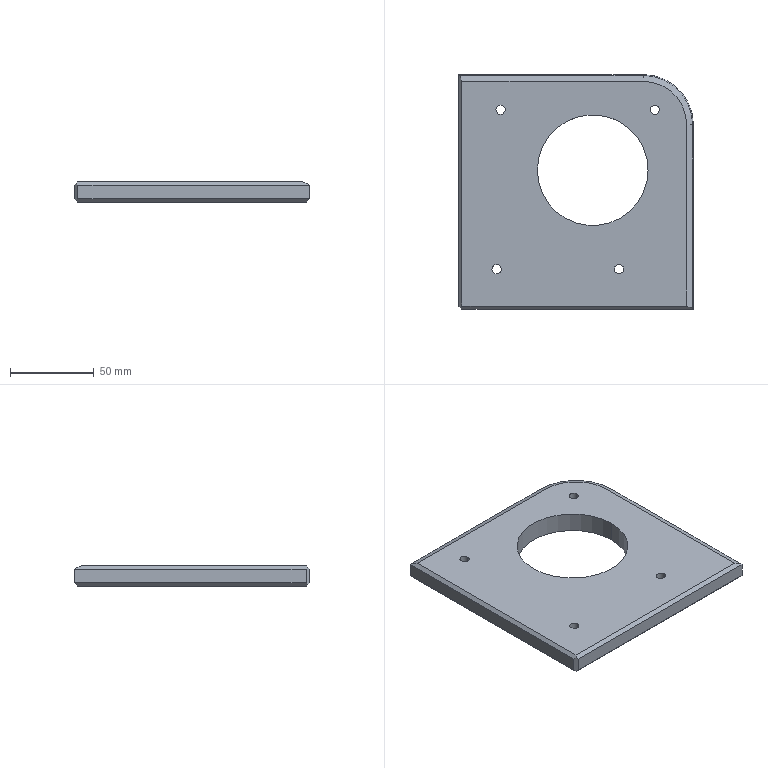Part | Creo | 1 solid | 43 faces | box 140 x 140 x 12 mm | volume 187002 mm3 | plane 21 | cylinder 19 | cone 3 | commonest cylinder face diameters 5.5 x8 9.5 x8 66 x2 60 x1
STEP:
#1=CARTESIAN_POINT('',(-313.,-373.005,1.));
#2=VERTEX_POINT('',#1);
#3=CARTESIAN_POINT('',(-313.,-239.005,1.));
#4=VERTEX_POINT('',#3);
#5=CARTESIAN_POINT('',(-313.,-373.005,1.));
#6=DIRECTION('',(0.,1.,0.));
#7=VECTOR('',#6,134.);
#8=LINE('',#5,#7);
#9=EDGE_CURVE('',#2,#4,#8,.T.);
#10=ORIENTED_EDGE('',*,*,#9,.T.);
#11=CARTESIAN_POINT('',(-205.,-239.005,1.));
#12=VERTEX_POINT('',#11);
#13=CARTESIAN_POINT('',(-313.,-239.005,1.));
#14=DIRECTION('',(1.,0.,0.));
#15=VECTOR('',#14,108.);
#16=LINE('',#13,#15);
#17=EDGE_CURVE('',#4,#12,#16,.T.);
#18=ORIENTED_EDGE('',*,*,#17,.T.);
#19=CARTESIAN_POINT('',(-179.,-265.005,1.));
#20=VERTEX_POINT('',#19);
#21=CARTESIAN_POINT('',(-205.,-265.005,1.));
#22=DIRECTION('',(0.,0.,1.));
#23=DIRECTION('',(1.,0.,0.));
#24=AXIS2_PLACEMENT_3D('',#21,#22,#23);
#25=CIRCLE('',#24,26.);
#26=EDGE_CURVE('',#20,#12,#25,.T.);
#27=ORIENTED_EDGE('',*,*,#26,.F.);
#28=CARTESIAN_POINT('',(-179.,-373.005,1.));
#29=VERTEX_POINT('',#28);
#30=CARTESIAN_POINT('',(-179.,-265.005,1.));
#31=DIRECTION('',(0.,-1.,0.));
#32=VECTOR('',#31,108.);
#33=LINE('',#30,#32);
#34=EDGE_CURVE('',#20,#29,#33,.T.);
#35=ORIENTED_EDGE('',*,*,#34,.T.);
#36=CARTESIAN_POINT('',(-179.,-373.005,1.));
#37=DIRECTION('',(-1.,0.,0.));
#38=VECTOR('',#37,134.);
#39=LINE('',#36,#38);
#40=EDGE_CURVE('',#29,#2,#39,.T.);
#41=ORIENTED_EDGE('',*,*,#40,.T.);
#42=EDGE_LOOP('',(#10,#18,#27,#35,#41));
#43=FACE_OUTER_BOUND('',#42,.F.);
#44=CARTESIAN_POINT('',(-295.118,-351.009,1.));
#45=VERTEX_POINT('',#44);
#46=CARTESIAN_POINT('',(-289.618,-351.009,1.));
#47=VERTEX_POINT('',#46);
#48=CARTESIAN_POINT('',(-292.368,-351.009,1.));
#49=DIRECTION('',(0.,0.,-1.));
#50=DIRECTION('',(-1.,0.,0.));
#51=AXIS2_PLACEMENT_3D('',#48,#49,#50);
#52=CIRCLE('',#51,2.75);
#53=EDGE_CURVE('',#45,#47,#52,.T.);
#54=ORIENTED_EDGE('',*,*,#53,.F.);
#55=CARTESIAN_POINT('',(-292.368,-351.009,1.));
#56=DIRECTION('',(0.,0.,-1.));
#57=DIRECTION('',(1.,0.,0.));
#58=AXIS2_PLACEMENT_3D('',#55,#56,#57);
#59=CIRCLE('',#58,2.75);
#60=EDGE_CURVE('',#47,#45,#59,.T.);
#61=ORIENTED_EDGE('',*,*,#60,.F.);
#62=EDGE_LOOP('',(#54,#61));
#63=FACE_BOUND('',#62,.F.);
#64=CARTESIAN_POINT('',(-200.75,-256.009,1.));
#65=VERTEX_POINT('',#64);
#66=CARTESIAN_POINT('',(-195.25,-256.009,1.));
#67=VERTEX_POINT('',#66);
#68=CARTESIAN_POINT('',(-198.,-256.009,1.));
#69=DIRECTION('',(0.,0.,-1.));
#70=DIRECTION('',(-1.,0.,0.));
#71=AXIS2_PLACEMENT_3D('',#68,#69,#70);
#72=CIRCLE('',#71,2.75);
#73=EDGE_CURVE('',#65,#67,#72,.T.);
#74=ORIENTED_EDGE('',*,*,#73,.F.);
#75=CARTESIAN_POINT('',(-198.,-256.009,1.));
#76=DIRECTION('',(0.,0.,-1.));
#77=DIRECTION('',(1.,0.,0.));
#78=AXIS2_PLACEMENT_3D('',#75,#76,#77);
#79=CIRCLE('',#78,2.75);
#80=EDGE_CURVE('',#67,#65,#79,.T.);
#81=ORIENTED_EDGE('',*,*,#80,.F.);
#82=EDGE_LOOP('',(#74,#81));
#83=FACE_BOUND('',#82,.F.);
#84=CARTESIAN_POINT('',(-202.,-292.005,1.));
#85=VERTEX_POINT('',#84);
#86=CARTESIAN_POINT('',(-268.,-292.005,1.));
#87=VERTEX_POINT('',#86);
#88=CARTESIAN_POINT('',(-235.,-292.005,1.));
#89=DIRECTION('',(0.,0.,-1.));
#90=DIRECTION('',(1.,0.,0.));
#91=AXIS2_PLACEMENT_3D('',#88,#89,#90);
#92=CIRCLE('',#91,33.);
#93=EDGE_CURVE('',#85,#87,#92,.T.);
#94=ORIENTED_EDGE('',*,*,#93,.F.);
#95=CARTESIAN_POINT('',(-235.,-292.005,1.));
#96=DIRECTION('',(0.,0.,-1.));
#97=DIRECTION('',(-1.,0.,0.));
#98=AXIS2_PLACEMENT_3D('',#95,#96,#97);
#99=CIRCLE('',#98,33.);
#100=EDGE_CURVE('',#87,#85,#99,.T.);
#101=ORIENTED_EDGE('',*,*,#100,.F.);
#102=EDGE_LOOP('',(#94,#101));
#103=FACE_BOUND('',#102,.F.);
#104=CARTESIAN_POINT('',(-292.75,-256.009,1.));
#105=VERTEX_POINT('',#104);
#106=CARTESIAN_POINT('',(-287.25,-256.009,1.));
#107=VERTEX_POINT('',#106);
#108=CARTESIAN_POINT('',(-290.,-256.009,1.));
#109=DIRECTION('',(0.,0.,-1.));
#110=DIRECTION('',(-1.,0.,0.));
#111=AXIS2_PLACEMENT_3D('',#108,#109,#110);
#112=CIRCLE('',#111,2.75);
#113=EDGE_CURVE('',#105,#107,#112,.T.);
#114=ORIENTED_EDGE('',*,*,#113,.F.);
#115=CARTESIAN_POINT('',(-290.,-256.009,1.));
#116=DIRECTION('',(0.,0.,-1.));
#117=DIRECTION('',(1.,0.,0.));
#118=AXIS2_PLACEMENT_3D('',#115,#116,#117);
#119=CIRCLE('',#118,2.75);
#120=EDGE_CURVE('',#107,#105,#119,.T.);
#121=ORIENTED_EDGE('',*,*,#120,.F.);
#122=EDGE_LOOP('',(#114,#121));
#123=FACE_BOUND('',#122,.F.);
#124=CARTESIAN_POINT('',(-222.118,-351.009,1.));
#125=VERTEX_POINT('',#124);
#126=CARTESIAN_POINT('',(-216.618,-351.009,1.));
#127=VERTEX_POINT('',#126);
#128=CARTESIAN_POINT('',(-219.368,-351.009,1.));
#129=DIRECTION('',(0.,0.,-1.));
#130=DIRECTION('',(-1.,0.,0.));
#131=AXIS2_PLACEMENT_3D('',#128,#129,#130);
#132=CIRCLE('',#131,2.75);
#133=EDGE_CURVE('',#125,#127,#132,.T.);
#134=ORIENTED_EDGE('',*,*,#133,.F.);
#135=CARTESIAN_POINT('',(-219.368,-351.009,1.));
#136=DIRECTION('',(0.,0.,-1.));
#137=DIRECTION('',(1.,0.,0.));
#138=AXIS2_PLACEMENT_3D('',#135,#136,#137);
#139=CIRCLE('',#138,2.75);
#140=EDGE_CURVE('',#127,#125,#139,.T.);
#141=ORIENTED_EDGE('',*,*,#140,.F.);
#142=EDGE_LOOP('',(#134,#141));
#143=FACE_BOUND('',#142,.F.);
#144=CARTESIAN_POINT('',(-245.,-302.505,1.));
#145=DIRECTION('',(0.,0.,1.));
#146=DIRECTION('',(1.,0.,0.));
#147=AXIS2_PLACEMENT_3D('',#144,#145,#146);
#148=PLANE('',#147);
#149=ADVANCED_FACE('',(#43,#63,#83,#103,#123,#143),#148,.T.);
#150=CARTESIAN_POINT('',(-315.,-235.005,-1.));
#151=VERTEX_POINT('',#150);
#152=CARTESIAN_POINT('',(-315.,-373.005,-1.));
#153=VERTEX_POINT('',#152);
#154=CARTESIAN_POINT('',(-315.,-235.005,-1.));
#155=DIRECTION('',(0.,-1.,0.));
#156=VECTOR('',#155,138.);
#157=LINE('',#154,#156);
#158=EDGE_CURVE('',#151,#153,#157,.T.);
#159=ORIENTED_EDGE('',*,*,#158,.F.);
#160=CARTESIAN_POINT('',(-314.414,-235.59,-0.4142));
#161=VERTEX_POINT('',#160);
#162=CARTESIAN_POINT('',(-314.414,-235.59,-0.4142));
#163=DIRECTION('',(-0.5774,0.5774,-0.5774));
#164=VECTOR('',#163,1.015);
#165=LINE('',#162,#164);
#166=EDGE_CURVE('',#161,#151,#165,.T.);
#167=ORIENTED_EDGE('',*,*,#166,.F.);
#168=CARTESIAN_POINT('',(-314.414,-235.59,-0.4142));
#169=DIRECTION('',(0.3574,-0.8629,0.3574));
#170=VECTOR('',#169,3.957);
#171=LINE('',#168,#170);
#172=EDGE_CURVE('',#161,#4,#171,.T.);
#173=ORIENTED_EDGE('',*,*,#172,.T.);
#174=ORIENTED_EDGE('',*,*,#9,.F.);
#175=CARTESIAN_POINT('',(-314.,-374.005,0.));
#176=VERTEX_POINT('',#175);
#177=CARTESIAN_POINT('',(-314.,-374.005,0.));
#178=DIRECTION('',(0.5774,0.5774,0.5774));
#179=VECTOR('',#178,1.732);
#180=LINE('',#177,#179);
#181=EDGE_CURVE('',#176,#2,#180,.T.);
#182=ORIENTED_EDGE('',*,*,#181,.F.);
#183=CARTESIAN_POINT('',(-315.,-373.005,-1.));
#184=DIRECTION('',(0.5774,-0.5774,0.5774));
#185=VECTOR('',#184,1.732);
#186=LINE('',#183,#185);
#187=EDGE_CURVE('',#153,#176,#186,.T.);
#188=ORIENTED_EDGE('',*,*,#187,.F.);
#189=EDGE_LOOP('',(#159,#167,#173,#174,#182,#188));
#190=FACE_OUTER_BOUND('',#189,.F.);
#191=CARTESIAN_POINT('',(-313.,-302.505,1.));
#192=DIRECTION('',(-0.7071,0.,0.7071));
#193=DIRECTION('',(0.,1.,0.));
#194=AXIS2_PLACEMENT_3D('',#191,#192,#193);
#195=PLANE('',#194);
#196=ADVANCED_FACE('',(#190),#195,.T.);
#197=CARTESIAN_POINT('',(-315.,-373.005,-9.));
#198=VERTEX_POINT('',#197);
#199=CARTESIAN_POINT('',(-315.,-373.005,-1.));
#200=DIRECTION('',(0.,0.,-1.));
#201=VECTOR('',#200,8.);
#202=LINE('',#199,#201);
#203=EDGE_CURVE('',#153,#198,#202,.T.);
#204=ORIENTED_EDGE('',*,*,#203,.T.);
#205=CARTESIAN_POINT('',(-315.,-235.005,-9.));
#206=VERTEX_POINT('',#205);
#207=CARTESIAN_POINT('',(-315.,-373.005,-9.));
#208=DIRECTION('',(0.,1.,0.));
#209=VECTOR('',#208,138.);
#210=LINE('',#207,#209);
#211=EDGE_CURVE('',#198,#206,#210,.T.);
#212=ORIENTED_EDGE('',*,*,#211,.T.);
#213=CARTESIAN_POINT('',(-315.,-235.005,-1.));
#214=DIRECTION('',(0.,0.,-1.));
#215=VECTOR('',#214,8.);
#216=LINE('',#213,#215);
#217=EDGE_CURVE('',#151,#206,#216,.T.);
#218=ORIENTED_EDGE('',*,*,#217,.F.);
#219=ORIENTED_EDGE('',*,*,#158,.T.);
#220=EDGE_LOOP('',(#204,#212,#218,#219));
#221=FACE_OUTER_BOUND('',#220,.F.);
#222=CARTESIAN_POINT('',(-315.,-0.004699,0.));
#223=DIRECTION('',(1.,0.,0.));
#224=DIRECTION('',(0.,-1.,0.));
#225=AXIS2_PLACEMENT_3D('',#222,#223,#224);
#226=PLANE('',#225);
#227=ADVANCED_FACE('',(#221),#226,.F.);
#228=CARTESIAN_POINT('',(-313.,-375.005,-9.));
#229=VERTEX_POINT('',#228);
#230=CARTESIAN_POINT('',(-313.,-375.005,-1.));
#231=VERTEX_POINT('',#230);
#232=CARTESIAN_POINT('',(-313.,-375.005,-9.));
#233=DIRECTION('',(0.,0.,1.));
#234=VECTOR('',#233,8.);
#235=LINE('',#232,#234);
#236=EDGE_CURVE('',#229,#231,#235,.T.);
#237=ORIENTED_EDGE('',*,*,#236,.F.);
#238=CARTESIAN_POINT('',(-314.,-374.005,-10.));
#239=VERTEX_POINT('',#238);
#240=CARTESIAN_POINT('',(-314.,-374.005,-10.));
#241=DIRECTION('',(0.5774,-0.5774,0.5774));
#242=VECTOR('',#241,1.732);
#243=LINE('',#240,#242);
#244=EDGE_CURVE('',#239,#229,#243,.T.);
#245=ORIENTED_EDGE('',*,*,#244,.F.);
#246=CARTESIAN_POINT('',(-315.,-373.005,-9.));
#247=DIRECTION('',(0.5774,-0.5774,-0.5774));
#248=VECTOR('',#247,1.732);
#249=LINE('',#246,#248);
#250=EDGE_CURVE('',#198,#239,#249,.T.);
#251=ORIENTED_EDGE('',*,*,#250,.F.);
#252=ORIENTED_EDGE('',*,*,#203,.F.);
#253=ORIENTED_EDGE('',*,*,#187,.T.);
#254=CARTESIAN_POINT('',(-314.,-374.005,0.));
#255=DIRECTION('',(0.5774,-0.5774,-0.5774));
#256=VECTOR('',#255,1.732);
#257=LINE('',#254,#256);
#258=EDGE_CURVE('',#176,#231,#257,.T.);
#259=ORIENTED_EDGE('',*,*,#258,.T.);
#260=EDGE_LOOP('',(#237,#245,#251,#252,#253,#259));
#261=FACE_OUTER_BOUND('',#260,.F.);
#262=CARTESIAN_POINT('',(-315.,-373.005,0.));
#263=DIRECTION('',(-0.7071,-0.7071,0.));
#264=DIRECTION('',(0.,0.,-1.));
#265=AXIS2_PLACEMENT_3D('',#262,#263,#264);
#266=PLANE('',#265);
#267=ADVANCED_FACE('',(#261),#266,.T.);
#268=CARTESIAN_POINT('',(-175.,-375.005,-1.));
#269=VERTEX_POINT('',#268);
#270=CARTESIAN_POINT('',(-175.,-375.005,-9.));
#271=VERTEX_POINT('',#270);
#272=CARTESIAN_POINT('',(-175.,-375.005,-1.));
#273=DIRECTION('',(0.,0.,-1.));
#274=VECTOR('',#273,8.);
#275=LINE('',#272,#274);
#276=EDGE_CURVE('',#269,#271,#275,.T.);
#277=ORIENTED_EDGE('',*,*,#276,.T.);
#278=CARTESIAN_POINT('',(-175.,-375.005,-9.));
#279=DIRECTION('',(-1.,0.,0.));
#280=VECTOR('',#279,138.);
#281=LINE('',#278,#280);
#282=EDGE_CURVE('',#271,#229,#281,.T.);
#283=ORIENTED_EDGE('',*,*,#282,.T.);
#284=ORIENTED_EDGE('',*,*,#236,.T.);
#285=CARTESIAN_POINT('',(-313.,-375.005,-1.));
#286=DIRECTION('',(1.,0.,0.));
#287=VECTOR('',#286,138.);
#288=LINE('',#285,#287);
#289=EDGE_CURVE('',#231,#269,#288,.T.);
#290=ORIENTED_EDGE('',*,*,#289,.T.);
#291=EDGE_LOOP('',(#277,#283,#284,#290));
#292=FACE_OUTER_BOUND('',#291,.F.);
#293=CARTESIAN_POINT('',(-265.,-375.005,165.));
#294=DIRECTION('',(0.,-1.,0.));
#295=DIRECTION('',(0.,0.,-1.));
#296=AXIS2_PLACEMENT_3D('',#293,#294,#295);
#297=PLANE('',#296);
#298=ADVANCED_FACE('',(#292),#297,.T.);
#299=ORIENTED_EDGE('',*,*,#276,.F.);
#300=CARTESIAN_POINT('',(-175.,-265.005,-1.));
#301=VERTEX_POINT('',#300);
#302=CARTESIAN_POINT('',(-175.,-375.005,-1.));
#303=DIRECTION('',(0.,1.,0.));
#304=VECTOR('',#303,110.);
#305=LINE('',#302,#304);
#306=EDGE_CURVE('',#269,#301,#305,.T.);
#307=ORIENTED_EDGE('',*,*,#306,.T.);
#308=CARTESIAN_POINT('',(-175.,-265.005,-9.));
#309=VERTEX_POINT('',#308);
#310=CARTESIAN_POINT('',(-175.,-265.005,-1.));
#311=DIRECTION('',(0.,0.,-1.));
#312=VECTOR('',#311,8.);
#313=LINE('',#310,#312);
#314=EDGE_CURVE('',#301,#309,#313,.T.);
#315=ORIENTED_EDGE('',*,*,#314,.T.);
#316=CARTESIAN_POINT('',(-175.,-265.005,-9.));
#317=DIRECTION('',(0.,-1.,0.));
#318=VECTOR('',#317,110.);
#319=LINE('',#316,#318);
#320=EDGE_CURVE('',#309,#271,#319,.T.);
#321=ORIENTED_EDGE('',*,*,#320,.T.);
#322=EDGE_LOOP('',(#299,#307,#315,#321));
#323=FACE_OUTER_BOUND('',#322,.F.);
#324=CARTESIAN_POINT('',(-175.,-302.505,-11.));
#325=DIRECTION('',(1.,0.,0.));
#326=DIRECTION('',(0.,0.,-1.));
#327=AXIS2_PLACEMENT_3D('',#324,#325,#326);
#328=PLANE('',#327);
#329=ADVANCED_FACE('',(#323),#328,.T.);
#330=CARTESIAN_POINT('',(-175.586,-374.419,-0.4142));
#331=VERTEX_POINT('',#330);
#332=CARTESIAN_POINT('',(-175.586,-265.005,-0.4142));
#333=VERTEX_POINT('',#332);
#334=CARTESIAN_POINT('',(-175.586,-374.419,-0.4142));
#335=DIRECTION('',(0.,1.,0.));
#336=VECTOR('',#335,109.414);
#337=LINE('',#334,#336);
#338=EDGE_CURVE('',#331,#333,#337,.T.);
#339=ORIENTED_EDGE('',*,*,#338,.T.);
#340=CARTESIAN_POINT('',(-175.586,-265.005,-0.4142));
#341=DIRECTION('',(0.7071,0.,-0.7071));
#342=VECTOR('',#341,0.8284);
#343=LINE('',#340,#342);
#344=EDGE_CURVE('',#333,#301,#343,.T.);
#345=ORIENTED_EDGE('',*,*,#344,.T.);
#346=ORIENTED_EDGE('',*,*,#306,.F.);
#347=CARTESIAN_POINT('',(-175.,-375.005,-1.));
#348=DIRECTION('',(-0.5774,0.5774,0.5774));
#349=VECTOR('',#348,1.015);
#350=LINE('',#347,#349);
#351=EDGE_CURVE('',#269,#331,#350,.T.);
#352=ORIENTED_EDGE('',*,*,#351,.T.);
#353=EDGE_LOOP('',(#339,#345,#346,#352));
#354=FACE_OUTER_BOUND('',#353,.F.);
#355=CARTESIAN_POINT('',(-175.,-302.505,-1.));
#356=DIRECTION('',(-0.7071,0.,-0.7071));
#357=DIRECTION('',(0.,-1.,0.));
#358=AXIS2_PLACEMENT_3D('',#355,#356,#357);
#359=PLANE('',#358);
#360=ADVANCED_FACE('',(#354),#359,.F.);
#361=CARTESIAN_POINT('',(-179.,-265.005,1.));
#362=DIRECTION('',(0.9239,0.,-0.3827));
#363=VECTOR('',#362,3.696);
#364=LINE('',#361,#363);
#365=EDGE_CURVE('',#20,#333,#364,.T.);
#366=ORIENTED_EDGE('',*,*,#365,.T.);
#367=ORIENTED_EDGE('',*,*,#338,.F.);
#368=CARTESIAN_POINT('',(-179.,-373.005,1.));
#369=DIRECTION('',(0.8629,-0.3574,-0.3574));
#370=VECTOR('',#369,3.957);
#371=LINE('',#368,#370);
#372=EDGE_CURVE('',#29,#331,#371,.T.);
#373=ORIENTED_EDGE('',*,*,#372,.F.);
#374=ORIENTED_EDGE('',*,*,#34,.F.);
#375=EDGE_LOOP('',(#366,#367,#373,#374));
#376=FACE_OUTER_BOUND('',#375,.F.);
#377=CARTESIAN_POINT('',(-179.,-302.505,1.));
#378=DIRECTION('',(0.3827,0.,0.9239));
#379=DIRECTION('',(0.,-1.,0.));
#380=AXIS2_PLACEMENT_3D('',#377,#378,#379);
#381=PLANE('',#380);
#382=ADVANCED_FACE('',(#376),#381,.T.);
#383=ORIENTED_EDGE('',*,*,#365,.F.);
#384=ORIENTED_EDGE('',*,*,#26,.T.);
#385=CARTESIAN_POINT('',(-205.,-235.59,-0.4142));
#386=VERTEX_POINT('',#385);
#387=CARTESIAN_POINT('',(-205.,-235.59,-0.4142));
#388=DIRECTION('',(0.,-0.9239,0.3827));
#389=VECTOR('',#388,3.696);
#390=LINE('',#387,#389);
#391=EDGE_CURVE('',#386,#12,#390,.T.);
#392=ORIENTED_EDGE('',*,*,#391,.F.);
#393=CARTESIAN_POINT('',(-205.,-265.005,-0.4142));
#394=DIRECTION('',(0.,0.,1.));
#395=DIRECTION('',(1.,0.,0.));
#396=AXIS2_PLACEMENT_3D('',#393,#394,#395);
#397=CIRCLE('',#396,29.414);
#398=EDGE_CURVE('',#333,#386,#397,.T.);
#399=ORIENTED_EDGE('',*,*,#398,.F.);
#400=EDGE_LOOP('',(#383,#384,#392,#399));
#401=FACE_OUTER_BOUND('',#400,.F.);
#402=CARTESIAN_POINT('',(-205.,-265.005,0.2929));
#403=DIRECTION('',(0.,0.,-1.));
#404=DIRECTION('',(-1.,0.,0.));
#405=AXIS2_PLACEMENT_3D('',#402,#403,#404);
#406=CONICAL_SURFACE('',#405,27.707,67.5);
#407=ADVANCED_FACE('',(#401),#406,.T.);
#408=ORIENTED_EDGE('',*,*,#391,.T.);
#409=ORIENTED_EDGE('',*,*,#17,.F.);
#410=ORIENTED_EDGE('',*,*,#172,.F.);
#411=CARTESIAN_POINT('',(-205.,-235.59,-0.4142));
#412=DIRECTION('',(-1.,0.,0.));
#413=VECTOR('',#412,109.414);
#414=LINE('',#411,#413);
#415=EDGE_CURVE('',#386,#161,#414,.T.);
#416=ORIENTED_EDGE('',*,*,#415,.F.);
#417=EDGE_LOOP('',(#408,#409,#410,#416));
#418=FACE_OUTER_BOUND('',#417,.F.);
#419=CARTESIAN_POINT('',(-245.,-239.005,1.));
#420=DIRECTION('',(0.,0.3827,0.9239));
#421=DIRECTION('',(1.,0.,0.));
#422=AXIS2_PLACEMENT_3D('',#419,#420,#421);
#423=PLANE('',#422);
#424=ADVANCED_FACE('',(#418),#423,.T.);
#425=ORIENTED_EDGE('',*,*,#166,.T.);
#426=CARTESIAN_POINT('',(-205.,-235.005,-1.));
#427=VERTEX_POINT('',#426);
#428=CARTESIAN_POINT('',(-205.,-235.005,-1.));
#429=DIRECTION('',(-1.,0.,0.));
#430=VECTOR('',#429,110.);
#431=LINE('',#428,#430);
#432=EDGE_CURVE('',#427,#151,#431,.T.);
#433=ORIENTED_EDGE('',*,*,#432,.F.);
#434=CARTESIAN_POINT('',(-205.,-235.005,-1.));
#435=DIRECTION('',(0.,-0.7071,0.7071));
#436=VECTOR('',#435,0.8284);
#437=LINE('',#434,#436);
#438=EDGE_CURVE('',#427,#386,#437,.T.);
#439=ORIENTED_EDGE('',*,*,#438,.T.);
#440=ORIENTED_EDGE('',*,*,#415,.T.);
#441=EDGE_LOOP('',(#425,#433,#439,#440));
#442=FACE_OUTER_BOUND('',#441,.F.);
#443=CARTESIAN_POINT('',(-245.,-235.005,-1.));
#444=DIRECTION('',(0.,-0.7071,-0.7071));
#445=DIRECTION('',(1.,0.,0.));
#446=AXIS2_PLACEMENT_3D('',#443,#444,#445);
#447=PLANE('',#446);
#448=ADVANCED_FACE('',(#442),#447,.F.);
#449=CARTESIAN_POINT('',(-205.,-235.005,-9.));
#450=VERTEX_POINT('',#449);
#451=CARTESIAN_POINT('',(-205.,-235.005,-9.));
#452=DIRECTION('',(0.,0.,1.));
#453=VECTOR('',#452,8.);
#454=LINE('',#451,#453);
#455=EDGE_CURVE('',#450,#427,#454,.T.);
#456=ORIENTED_EDGE('',*,*,#455,.T.);
#457=ORIENTED_EDGE('',*,*,#432,.T.);
#458=ORIENTED_EDGE('',*,*,#217,.T.);
#459=CARTESIAN_POINT('',(-315.,-235.005,-9.));
#460=DIRECTION('',(1.,0.,0.));
#461=VECTOR('',#460,110.);
#462=LINE('',#459,#461);
#463=EDGE_CURVE('',#206,#450,#462,.T.);
#464=ORIENTED_EDGE('',*,*,#463,.T.);
#465=EDGE_LOOP('',(#456,#457,#458,#464));
#466=FACE_OUTER_BOUND('',#465,.F.);
#467=CARTESIAN_POINT('',(-245.,-235.005,-11.));
#468=DIRECTION('',(0.,1.,0.));
#469=DIRECTION('',(0.,0.,1.));
#470=AXIS2_PLACEMENT_3D('',#467,#468,#469);
#471=PLANE('',#470);
#472=ADVANCED_FACE('',(#466),#471,.T.);
#473=ORIENTED_EDGE('',*,*,#314,.F.);
#474=CARTESIAN_POINT('',(-205.,-265.005,-1.));
#475=DIRECTION('',(0.,0.,1.));
#476=DIRECTION('',(1.,0.,0.));
#477=AXIS2_PLACEMENT_3D('',#474,#475,#476);
#478=CIRCLE('',#477,30.);
#479=EDGE_CURVE('',#301,#427,#478,.T.);
#480=ORIENTED_EDGE('',*,*,#479,.T.);
#481=ORIENTED_EDGE('',*,*,#455,.F.);
#482=CARTESIAN_POINT('',(-205.,-265.005,-9.));
#483=DIRECTION('',(0.,0.,-1.));
#484=DIRECTION('',(0.,1.,0.));
#485=AXIS2_PLACEMENT_3D('',#482,#483,#484);
#486=CIRCLE('',#485,30.);
#487=EDGE_CURVE('',#450,#309,#486,.T.);
#488=ORIENTED_EDGE('',*,*,#487,.T.);
#489=EDGE_LOOP('',(#473,#480,#481,#488));
#490=FACE_OUTER_BOUND('',#489,.F.);
#491=CARTESIAN_POINT('',(-205.,-265.005,-11.));
#492=DIRECTION('',(0.,0.,1.));
#493=DIRECTION('',(1.,0.,0.));
#494=AXIS2_PLACEMENT_3D('',#491,#492,#493);
#495=CYLINDRICAL_SURFACE('',#494,30.);
#496=ADVANCED_FACE('',(#490),#495,.T.);
#497=ORIENTED_EDGE('',*,*,#438,.F.);
#498=ORIENTED_EDGE('',*,*,#479,.F.);
#499=ORIENTED_EDGE('',*,*,#344,.F.);
#500=ORIENTED_EDGE('',*,*,#398,.T.);
#501=EDGE_LOOP('',(#497,#498,#499,#500));
#502=FACE_OUTER_BOUND('',#501,.F.);
#503=CARTESIAN_POINT('',(-205.,-265.005,-0.7071));
#504=DIRECTION('',(0.,0.,-1.));
#505=DIRECTION('',(-1.,0.,0.));
#506=AXIS2_PLACEMENT_3D('',#503,#504,#505);
#507=CONICAL_SURFACE('',#506,29.707,45.);
#508=ADVANCED_FACE('',(#502),#507,.T.);
#509=CARTESIAN_POINT('',(-177.,-265.005,-11.));
#510=VERTEX_POINT('',#509);
#511=CARTESIAN_POINT('',(-175.,-265.005,-9.));
#512=DIRECTION('',(-0.7071,0.,-0.7071));
#513=VECTOR('',#512,2.828);
#514=LINE('',#511,#513);
#515=EDGE_CURVE('',#309,#510,#514,.T.);
#516=ORIENTED_EDGE('',*,*,#515,.F.);
#517=ORIENTED_EDGE('',*,*,#487,.F.);
#518=CARTESIAN_POINT('',(-205.,-237.005,-11.));
#519=VERTEX_POINT('',#518);
#520=CARTESIAN_POINT('',(-205.,-237.005,-11.));
#521=DIRECTION('',(0.,0.7071,0.7071));
#522=VECTOR('',#521,2.828);
#523=LINE('',#520,#522);
#524=EDGE_CURVE('',#519,#450,#523,.T.);
#525=ORIENTED_EDGE('',*,*,#524,.F.);
#526=CARTESIAN_POINT('',(-205.,-265.005,-11.));
#527=DIRECTION('',(0.,0.,-1.));
#528=DIRECTION('',(0.,1.,0.));
#529=AXIS2_PLACEMENT_3D('',#526,#527,#528);
#530=CIRCLE('',#529,28.);
#531=EDGE_CURVE('',#519,#510,#530,.T.);
#532=ORIENTED_EDGE('',*,*,#531,.T.);
#533=EDGE_LOOP('',(#516,#517,#525,#532));
#534=FACE_OUTER_BOUND('',#533,.F.);
#535=CARTESIAN_POINT('',(-205.,-265.005,-10.));
#536=DIRECTION('',(0.,0.,1.));
#537=DIRECTION('',(1.,0.,0.));
#538=AXIS2_PLACEMENT_3D('',#535,#536,#537);
#539=CONICAL_SURFACE('',#538,29.,45.);
#540=ADVANCED_FACE('',(#534),#539,.T.);
#541=CARTESIAN_POINT('',(-177.,-373.005,-11.));
#542=VERTEX_POINT('',#541);
#543=CARTESIAN_POINT('',(-175.,-375.005,-9.));
#544=DIRECTION('',(-0.5774,0.5774,-0.5774));
#545=VECTOR('',#544,3.464);
#546=LINE('',#543,#545);
#547=EDGE_CURVE('',#271,#542,#546,.T.);
#548=ORIENTED_EDGE('',*,*,#547,.F.);
#549=ORIENTED_EDGE('',*,*,#320,.F.);
#550=ORIENTED_EDGE('',*,*,#515,.T.);
#551=CARTESIAN_POINT('',(-177.,-373.005,-11.));
#552=DIRECTION('',(0.,1.,0.));
#553=VECTOR('',#552,108.);
#554=LINE('',#551,#553);
#555=EDGE_CURVE('',#542,#510,#554,.T.);
#556=ORIENTED_EDGE('',*,*,#555,.F.);
#557=EDGE_LOOP('',(#548,#549,#550,#556));
#558=FACE_OUTER_BOUND('',#557,.F.);
#559=CARTESIAN_POINT('',(-175.,-302.505,-9.));
#560=DIRECTION('',(-0.7071,0.,0.7071));
#561=DIRECTION('',(0.,1.,0.));
#562=AXIS2_PLACEMENT_3D('',#559,#560,#561);
#563=PLANE('',#562);
#564=ADVANCED_FACE('',(#558),#563,.F.);
#565=CARTESIAN_POINT('',(-313.,-373.005,-11.));
#566=VERTEX_POINT('',#565);
#567=CARTESIAN_POINT('',(-313.,-373.005,-11.));
#568=DIRECTION('',(1.,0.,0.));
#569=VECTOR('',#568,136.);
#570=LINE('',#567,#569);
#571=EDGE_CURVE('',#566,#542,#570,.T.);
#572=ORIENTED_EDGE('',*,*,#571,.F.);
#573=CARTESIAN_POINT('',(-313.,-373.005,-11.));
#574=DIRECTION('',(-0.5774,-0.5774,0.5774));
#575=VECTOR('',#574,1.732);
#576=LINE('',#573,#575);
#577=EDGE_CURVE('',#566,#239,#576,.T.);
#578=ORIENTED_EDGE('',*,*,#577,.T.);
#579=ORIENTED_EDGE('',*,*,#244,.T.);
#580=ORIENTED_EDGE('',*,*,#282,.F.);
#581=ORIENTED_EDGE('',*,*,#547,.T.);
#582=EDGE_LOOP('',(#572,#578,#579,#580,#581));
#583=FACE_OUTER_BOUND('',#582,.F.);
#584=CARTESIAN_POINT('',(-265.,-375.005,-9.));
#585=DIRECTION('',(0.,0.7071,0.7071));
#586=DIRECTION('',(1.,0.,0.));
#587=AXIS2_PLACEMENT_3D('',#584,#585,#586);
#588=PLANE('',#587);
#589=ADVANCED_FACE('',(#583),#588,.F.);
#590=CARTESIAN_POINT('',(-313.,-237.005,-11.));
#591=VERTEX_POINT('',#590);
#592=CARTESIAN_POINT('',(-313.,-237.005,-11.));
#593=DIRECTION('',(0.,-1.,0.));
#594=VECTOR('',#593,136.);
#595=LINE('',#592,#594);
#596=EDGE_CURVE('',#591,#566,#595,.T.);
#597=ORIENTED_EDGE('',*,*,#596,.T.);
#598=ORIENTED_EDGE('',*,*,#571,.T.);
#599=ORIENTED_EDGE('',*,*,#555,.T.);
#600=ORIENTED_EDGE('',*,*,#531,.F.);
#601=CARTESIAN_POINT('',(-205.,-237.005,-11.));
#602=DIRECTION('',(-1.,0.,0.));
#603=VECTOR('',#602,108.);
#604=LINE('',#601,#603);
#605=EDGE_CURVE('',#519,#591,#604,.T.);
#606=ORIENTED_EDGE('',*,*,#605,.T.);
#607=EDGE_LOOP('',(#597,#598,#599,#600,#606));
#608=FACE_OUTER_BOUND('',#607,.F.);
#609=CARTESIAN_POINT('',(-224.118,-351.009,-11.));
#610=VERTEX_POINT('',#609);
#611=CARTESIAN_POINT('',(-214.618,-351.009,-11.));
#612=VERTEX_POINT('',#611);
#613=CARTESIAN_POINT('',(-219.368,-351.009,-11.));
#614=DIRECTION('',(0.,0.,1.));
#615=DIRECTION('',(-1.,0.,0.));
#616=AXIS2_PLACEMENT_3D('',#613,#614,#615);
#617=CIRCLE('',#616,4.75);
#618=EDGE_CURVE('',#610,#612,#617,.T.);
#619=ORIENTED_EDGE('',*,*,#618,.F.);
#620=CARTESIAN_POINT('',(-219.368,-351.009,-11.));
#621=DIRECTION('',(0.,0.,1.));
#622=DIRECTION('',(1.,0.,0.));
#623=AXIS2_PLACEMENT_3D('',#620,#621,#622);
#624=CIRCLE('',#623,4.75);
#625=EDGE_CURVE('',#612,#610,#624,.T.);
#626=ORIENTED_EDGE('',*,*,#625,.F.);
#627=EDGE_LOOP('',(#619,#626));
#628=FACE_BOUND('',#627,.F.);
#629=CARTESIAN_POINT('',(-297.118,-351.009,-11.));
#630=VERTEX_POINT('',#629);
#631=CARTESIAN_POINT('',(-287.618,-351.009,-11.));
#632=VERTEX_POINT('',#631);
#633=CARTESIAN_POINT('',(-292.368,-351.009,-11.));
#634=DIRECTION('',(0.,0.,1.));
#635=DIRECTION('',(-1.,0.,0.));
#636=AXIS2_PLACEMENT_3D('',#633,#634,#635);
#637=CIRCLE('',#636,4.75);
#638=EDGE_CURVE('',#630,#632,#637,.T.);
#639=ORIENTED_EDGE('',*,*,#638,.F.);
#640=CARTESIAN_POINT('',(-292.368,-351.009,-11.));
#641=DIRECTION('',(0.,0.,1.));
#642=DIRECTION('',(1.,0.,0.));
#643=AXIS2_PLACEMENT_3D('',#640,#641,#642);
#644=CIRCLE('',#643,4.75);
#645=EDGE_CURVE('',#632,#630,#644,.T.);
#646=ORIENTED_EDGE('',*,*,#645,.F.);
#647=EDGE_LOOP('',(#639,#646));
#648=FACE_BOUND('',#647,.F.);
#649=CARTESIAN_POINT('',(-294.75,-256.009,-11.));
#650=VERTEX_POINT('',#649);
#651=CARTESIAN_POINT('',(-285.25,-256.009,-11.));
#652=VERTEX_POINT('',#651);
#653=CARTESIAN_POINT('',(-290.,-256.009,-11.));
#654=DIRECTION('',(0.,0.,1.));
#655=DIRECTION('',(-1.,0.,0.));
#656=AXIS2_PLACEMENT_3D('',#653,#654,#655);
#657=CIRCLE('',#656,4.75);
#658=EDGE_CURVE('',#650,#652,#657,.T.);
#659=ORIENTED_EDGE('',*,*,#658,.F.);
#660=CARTESIAN_POINT('',(-290.,-256.009,-11.));
#661=DIRECTION('',(0.,0.,1.));
#662=DIRECTION('',(1.,0.,0.));
#663=AXIS2_PLACEMENT_3D('',#660,#661,#662);
#664=CIRCLE('',#663,4.75);
#665=EDGE_CURVE('',#652,#650,#664,.T.);
#666=ORIENTED_EDGE('',*,*,#665,.F.);
#667=EDGE_LOOP('',(#659,#666));
#668=FACE_BOUND('',#667,.F.);
#669=CARTESIAN_POINT('',(-202.75,-256.009,-11.));
#670=VERTEX_POINT('',#669);
#671=CARTESIAN_POINT('',(-193.25,-256.009,-11.));
#672=VERTEX_POINT('',#671);
#673=CARTESIAN_POINT('',(-198.,-256.009,-11.));
#674=DIRECTION('',(0.,0.,1.));
#675=DIRECTION('',(-1.,0.,0.));
#676=AXIS2_PLACEMENT_3D('',#673,#674,#675);
#677=CIRCLE('',#676,4.75);
#678=EDGE_CURVE('',#670,#672,#677,.T.);
#679=ORIENTED_EDGE('',*,*,#678,.F.);
#680=CARTESIAN_POINT('',(-198.,-256.009,-11.));
#681=DIRECTION('',(0.,0.,1.));
#682=DIRECTION('',(1.,0.,0.));
#683=AXIS2_PLACEMENT_3D('',#680,#681,#682);
#684=CIRCLE('',#683,4.75);
#685=EDGE_CURVE('',#672,#670,#684,.T.);
#686=ORIENTED_EDGE('',*,*,#685,.F.);
#687=EDGE_LOOP('',(#679,#686));
#688=FACE_BOUND('',#687,.F.);
#689=CARTESIAN_POINT('',(-268.,-292.005,-11.));
#690=VERTEX_POINT('',#689);
#691=CARTESIAN_POINT('',(-202.,-292.005,-11.));
#692=VERTEX_POINT('',#691);
#693=CARTESIAN_POINT('',(-235.,-292.005,-11.));
#694=DIRECTION('',(0.,0.,1.));
#695=DIRECTION('',(-1.,0.,0.));
#696=AXIS2_PLACEMENT_3D('',#693,#694,#695);
#697=CIRCLE('',#696,33.);
#698=EDGE_CURVE('',#690,#692,#697,.T.);
#699=ORIENTED_EDGE('',*,*,#698,.F.);
#700=CARTESIAN_POINT('',(-235.,-292.005,-11.));
#701=DIRECTION('',(0.,0.,1.));
#702=DIRECTION('',(1.,0.,0.));
#703=AXIS2_PLACEMENT_3D('',#700,#701,#702);
#704=CIRCLE('',#703,33.);
#705=EDGE_CURVE('',#692,#690,#704,.T.);
#706=ORIENTED_EDGE('',*,*,#705,.F.);
#707=EDGE_LOOP('',(#699,#706));
#708=FACE_BOUND('',#707,.F.);
#709=CARTESIAN_POINT('',(-245.,-302.505,-11.));
#710=DIRECTION('',(0.,0.,-1.));
#711=DIRECTION('',(-1.,0.,0.));
#712=AXIS2_PLACEMENT_3D('',#709,#710,#711);
#713=PLANE('',#712);
#714=ADVANCED_FACE('',(#608,#628,#648,#668,#688,#708),#713,.T.);
#715=ORIENTED_EDGE('',*,*,#211,.F.);
#716=ORIENTED_EDGE('',*,*,#250,.T.);
#717=ORIENTED_EDGE('',*,*,#577,.F.);
#718=ORIENTED_EDGE('',*,*,#596,.F.);
#719=CARTESIAN_POINT('',(-313.,-237.005,-11.));
#720=DIRECTION('',(-0.5774,0.5774,0.5774));
#721=VECTOR('',#720,3.464);
#722=LINE('',#719,#721);
#723=EDGE_CURVE('',#591,#206,#722,.T.);
#724=ORIENTED_EDGE('',*,*,#723,.T.);
#725=EDGE_LOOP('',(#715,#716,#717,#718,#724));
#726=FACE_OUTER_BOUND('',#725,.F.);
#727=CARTESIAN_POINT('',(-315.,-0.004699,-9.));
#728=DIRECTION('',(-0.7071,0.,-0.7071));
#729=DIRECTION('',(0.,1.,0.));
#730=AXIS2_PLACEMENT_3D('',#727,#728,#729);
#731=PLANE('',#730);
#732=ADVANCED_FACE('',(#726),#731,.T.);
#733=ORIENTED_EDGE('',*,*,#524,.T.);
#734=ORIENTED_EDGE('',*,*,#463,.F.);
#735=ORIENTED_EDGE('',*,*,#723,.F.);
#736=ORIENTED_EDGE('',*,*,#605,.F.);
#737=EDGE_LOOP('',(#733,#734,#735,#736));
#738=FACE_OUTER_BOUND('',#737,.F.);
#739=CARTESIAN_POINT('',(-245.,-235.005,-9.));
#740=DIRECTION('',(0.,-0.7071,0.7071));
#741=DIRECTION('',(-1.,0.,0.));
#742=AXIS2_PLACEMENT_3D('',#739,#740,#741);
#743=PLANE('',#742);
#744=ADVANCED_FACE('',(#738),#743,.F.);
#745=CARTESIAN_POINT('',(-214.618,-351.009,-5.));
#746=VERTEX_POINT('',#745);
#747=CARTESIAN_POINT('',(-224.118,-351.009,-5.));
#748=VERTEX_POINT('',#747);
#749=CARTESIAN_POINT('',(-219.368,-351.009,-5.));
#750=DIRECTION('',(0.,0.,-1.));
#751=DIRECTION('',(1.,0.,0.));
#752=AXIS2_PLACEMENT_3D('',#749,#750,#751);
#753=CIRCLE('',#752,4.75);
#754=EDGE_CURVE('',#746,#748,#753,.T.);
#755=ORIENTED_EDGE('',*,*,#754,.T.);
#756=CARTESIAN_POINT('',(-224.118,-351.009,-5.));
#757=DIRECTION('',(0.,0.,-1.));
#758=VECTOR('',#757,6.);
#759=LINE('',#756,#758);
#760=EDGE_CURVE('',#748,#610,#759,.T.);
#761=ORIENTED_EDGE('',*,*,#760,.T.);
#762=ORIENTED_EDGE('',*,*,#618,.T.);
#763=CARTESIAN_POINT('',(-214.618,-351.009,-5.));
#764=DIRECTION('',(0.,0.,-1.));
#765=VECTOR('',#764,6.);
#766=LINE('',#763,#765);
#767=EDGE_CURVE('',#746,#612,#766,.T.);
#768=ORIENTED_EDGE('',*,*,#767,.F.);
#769=EDGE_LOOP('',(#755,#761,#762,#768));
#770=FACE_OUTER_BOUND('',#769,.F.);
#771=CARTESIAN_POINT('',(-219.368,-351.009,-11.));
#772=DIRECTION('',(0.,0.,-1.));
#773=DIRECTION('',(-1.,0.,0.));
#774=AXIS2_PLACEMENT_3D('',#771,#772,#773);
#775=CYLINDRICAL_SURFACE('',#774,4.75);
#776=ADVANCED_FACE('',(#770),#775,.F.);
#777=CARTESIAN_POINT('',(-219.368,-351.009,-5.));
#778=DIRECTION('',(0.,0.,-1.));
#779=DIRECTION('',(-1.,0.,0.));
#780=AXIS2_PLACEMENT_3D('',#777,#778,#779);
#781=CIRCLE('',#780,4.75);
#782=EDGE_CURVE('',#748,#746,#781,.T.);
#783=ORIENTED_EDGE('',*,*,#782,.F.);
#784=ORIENTED_EDGE('',*,*,#754,.F.);
#785=EDGE_LOOP('',(#783,#784));
#786=FACE_OUTER_BOUND('',#785,.F.);
#787=CARTESIAN_POINT('',(-222.118,-351.009,-5.));
#788=VERTEX_POINT('',#787);
#789=CARTESIAN_POINT('',(-216.618,-351.009,-5.));
#790=VERTEX_POINT('',#789);
#791=CARTESIAN_POINT('',(-219.368,-351.009,-5.));
#792=DIRECTION('',(0.,0.,1.));
#793=DIRECTION('',(-1.,0.,0.));
#794=AXIS2_PLACEMENT_3D('',#791,#792,#793);
#795=CIRCLE('',#794,2.75);
#796=EDGE_CURVE('',#788,#790,#795,.T.);
#797=ORIENTED_EDGE('',*,*,#796,.F.);
#798=CARTESIAN_POINT('',(-219.368,-351.009,-5.));
#799=DIRECTION('',(0.,0.,1.));
#800=DIRECTION('',(1.,0.,0.));
#801=AXIS2_PLACEMENT_3D('',#798,#799,#800);
#802=CIRCLE('',#801,2.75);
#803=EDGE_CURVE('',#790,#788,#802,.T.);
#804=ORIENTED_EDGE('',*,*,#803,.F.);
#805=EDGE_LOOP('',(#797,#804));
#806=FACE_BOUND('',#805,.F.);
#807=CARTESIAN_POINT('',(-219.368,-346.259,-5.));
#808=DIRECTION('',(0.,0.,1.));
#809=DIRECTION('',(1.,0.,0.));
#810=AXIS2_PLACEMENT_3D('',#807,#808,#809);
#811=PLANE('',#810);
#812=ADVANCED_FACE('',(#786,#806),#811,.F.);
#813=ORIENTED_EDGE('',*,*,#140,.T.);
#814=CARTESIAN_POINT('',(-222.118,-351.009,1.));
#815=DIRECTION('',(0.,0.,-1.));
#816=VECTOR('',#815,6.);
#817=LINE('',#814,#816);
#818=EDGE_CURVE('',#125,#788,#817,.T.);
#819=ORIENTED_EDGE('',*,*,#818,.T.);
#820=ORIENTED_EDGE('',*,*,#796,.T.);
#821=CARTESIAN_POINT('',(-216.618,-351.009,1.));
#822=DIRECTION('',(0.,0.,-1.));
#823=VECTOR('',#822,6.);
#824=LINE('',#821,#823);
#825=EDGE_CURVE('',#127,#790,#824,.T.);
#826=ORIENTED_EDGE('',*,*,#825,.F.);
#827=EDGE_LOOP('',(#813,#819,#820,#826));
#828=FACE_OUTER_BOUND('',#827,.F.);
#829=CARTESIAN_POINT('',(-219.368,-351.009,-11.));
#830=DIRECTION('',(0.,0.,-1.));
#831=DIRECTION('',(-1.,0.,0.));
#832=AXIS2_PLACEMENT_3D('',#829,#830,#831);
#833=CYLINDRICAL_SURFACE('',#832,2.75);
#834=ADVANCED_FACE('',(#828),#833,.F.);
#835=ORIENTED_EDGE('',*,*,#133,.T.);
#836=ORIENTED_EDGE('',*,*,#825,.T.);
#837=ORIENTED_EDGE('',*,*,#803,.T.);
#838=ORIENTED_EDGE('',*,*,#818,.F.);
#839=EDGE_LOOP('',(#835,#836,#837,#838));
#840=FACE_OUTER_BOUND('',#839,.F.);
#841=CARTESIAN_POINT('',(-219.368,-351.009,-11.));
#842=DIRECTION('',(0.,0.,-1.));
#843=DIRECTION('',(-1.,0.,0.));
#844=AXIS2_PLACEMENT_3D('',#841,#842,#843);
#845=CYLINDRICAL_SURFACE('',#844,2.75);
#846=ADVANCED_FACE('',(#840),#845,.F.);
#847=ORIENTED_EDGE('',*,*,#782,.T.);
#848=ORIENTED_EDGE('',*,*,#767,.T.);
#849=ORIENTED_EDGE('',*,*,#625,.T.);
#850=ORIENTED_EDGE('',*,*,#760,.F.);
#851=EDGE_LOOP('',(#847,#848,#849,#850));
#852=FACE_OUTER_BOUND('',#851,.F.);
#853=CARTESIAN_POINT('',(-219.368,-351.009,-11.));
#854=DIRECTION('',(0.,0.,-1.));
#855=DIRECTION('',(-1.,0.,0.));
#856=AXIS2_PLACEMENT_3D('',#853,#854,#855);
#857=CYLINDRICAL_SURFACE('',#856,4.75);
#858=ADVANCED_FACE('',(#852),#857,.F.);
#859=CARTESIAN_POINT('',(-287.618,-351.009,-5.));
#860=VERTEX_POINT('',#859);
#861=CARTESIAN_POINT('',(-297.118,-351.009,-5.));
#862=VERTEX_POINT('',#861);
#863=CARTESIAN_POINT('',(-292.368,-351.009,-5.));
#864=DIRECTION('',(0.,0.,-1.));
#865=DIRECTION('',(1.,0.,0.));
#866=AXIS2_PLACEMENT_3D('',#863,#864,#865);
#867=CIRCLE('',#866,4.75);
#868=EDGE_CURVE('',#860,#862,#867,.T.);
#869=ORIENTED_EDGE('',*,*,#868,.T.);
#870=CARTESIAN_POINT('',(-297.118,-351.009,-5.));
#871=DIRECTION('',(0.,0.,-1.));
#872=VECTOR('',#871,6.);
#873=LINE('',#870,#872);
#874=EDGE_CURVE('',#862,#630,#873,.T.);
#875=ORIENTED_EDGE('',*,*,#874,.T.);
#876=ORIENTED_EDGE('',*,*,#638,.T.);
#877=CARTESIAN_POINT('',(-287.618,-351.009,-5.));
#878=DIRECTION('',(0.,0.,-1.));
#879=VECTOR('',#878,6.);
#880=LINE('',#877,#879);
#881=EDGE_CURVE('',#860,#632,#880,.T.);
#882=ORIENTED_EDGE('',*,*,#881,.F.);
#883=EDGE_LOOP('',(#869,#875,#876,#882));
#884=FACE_OUTER_BOUND('',#883,.F.);
#885=CARTESIAN_POINT('',(-292.368,-351.009,-11.));
#886=DIRECTION('',(0.,0.,-1.));
#887=DIRECTION('',(-1.,0.,0.));
#888=AXIS2_PLACEMENT_3D('',#885,#886,#887);
#889=CYLINDRICAL_SURFACE('',#888,4.75);
#890=ADVANCED_FACE('',(#884),#889,.F.);
#891=CARTESIAN_POINT('',(-292.368,-351.009,-5.));
#892=DIRECTION('',(0.,0.,-1.));
#893=DIRECTION('',(-1.,0.,0.));
#894=AXIS2_PLACEMENT_3D('',#891,#892,#893);
#895=CIRCLE('',#894,4.75);
#896=EDGE_CURVE('',#862,#860,#895,.T.);
#897=ORIENTED_EDGE('',*,*,#896,.F.);
#898=ORIENTED_EDGE('',*,*,#868,.F.);
#899=EDGE_LOOP('',(#897,#898));
#900=FACE_OUTER_BOUND('',#899,.F.);
#901=CARTESIAN_POINT('',(-295.118,-351.009,-5.));
#902=VERTEX_POINT('',#901);
#903=CARTESIAN_POINT('',(-289.618,-351.009,-5.));
#904=VERTEX_POINT('',#903);
#905=CARTESIAN_POINT('',(-292.368,-351.009,-5.));
#906=DIRECTION('',(0.,0.,1.));
#907=DIRECTION('',(-1.,0.,0.));
#908=AXIS2_PLACEMENT_3D('',#905,#906,#907);
#909=CIRCLE('',#908,2.75);
#910=EDGE_CURVE('',#902,#904,#909,.T.);
#911=ORIENTED_EDGE('',*,*,#910,.F.);
#912=CARTESIAN_POINT('',(-292.368,-351.009,-5.));
#913=DIRECTION('',(0.,0.,1.));
#914=DIRECTION('',(1.,0.,0.));
#915=AXIS2_PLACEMENT_3D('',#912,#913,#914);
#916=CIRCLE('',#915,2.75);
#917=EDGE_CURVE('',#904,#902,#916,.T.);
#918=ORIENTED_EDGE('',*,*,#917,.F.);
#919=EDGE_LOOP('',(#911,#918));
#920=FACE_BOUND('',#919,.F.);
#921=CARTESIAN_POINT('',(-292.368,-346.259,-5.));
#922=DIRECTION('',(0.,0.,1.));
#923=DIRECTION('',(1.,0.,0.));
#924=AXIS2_PLACEMENT_3D('',#921,#922,#923);
#925=PLANE('',#924);
#926=ADVANCED_FACE('',(#900,#920),#925,.F.);
#927=ORIENTED_EDGE('',*,*,#60,.T.);
#928=CARTESIAN_POINT('',(-295.118,-351.009,1.));
#929=DIRECTION('',(0.,0.,-1.));
#930=VECTOR('',#929,6.);
#931=LINE('',#928,#930);
#932=EDGE_CURVE('',#45,#902,#931,.T.);
#933=ORIENTED_EDGE('',*,*,#932,.T.);
#934=ORIENTED_EDGE('',*,*,#910,.T.);
#935=CARTESIAN_POINT('',(-289.618,-351.009,1.));
#936=DIRECTION('',(0.,0.,-1.));
#937=VECTOR('',#936,6.);
#938=LINE('',#935,#937);
#939=EDGE_CURVE('',#47,#904,#938,.T.);
#940=ORIENTED_EDGE('',*,*,#939,.F.);
#941=EDGE_LOOP('',(#927,#933,#934,#940));
#942=FACE_OUTER_BOUND('',#941,.F.);
#943=CARTESIAN_POINT('',(-292.368,-351.009,-11.));
#944=DIRECTION('',(0.,0.,-1.));
#945=DIRECTION('',(-1.,0.,0.));
#946=AXIS2_PLACEMENT_3D('',#943,#944,#945);
#947=CYLINDRICAL_SURFACE('',#946,2.75);
#948=ADVANCED_FACE('',(#942),#947,.F.);
#949=ORIENTED_EDGE('',*,*,#53,.T.);
#950=ORIENTED_EDGE('',*,*,#939,.T.);
#951=ORIENTED_EDGE('',*,*,#917,.T.);
#952=ORIENTED_EDGE('',*,*,#932,.F.);
#953=EDGE_LOOP('',(#949,#950,#951,#952));
#954=FACE_OUTER_BOUND('',#953,.F.);
#955=CARTESIAN_POINT('',(-292.368,-351.009,-11.));
#956=DIRECTION('',(0.,0.,-1.));
#957=DIRECTION('',(-1.,0.,0.));
#958=AXIS2_PLACEMENT_3D('',#955,#956,#957);
#959=CYLINDRICAL_SURFACE('',#958,2.75);
#960=ADVANCED_FACE('',(#954),#959,.F.);
#961=ORIENTED_EDGE('',*,*,#896,.T.);
#962=ORIENTED_EDGE('',*,*,#881,.T.);
#963=ORIENTED_EDGE('',*,*,#645,.T.);
#964=ORIENTED_EDGE('',*,*,#874,.F.);
#965=EDGE_LOOP('',(#961,#962,#963,#964));
#966=FACE_OUTER_BOUND('',#965,.F.);
#967=CARTESIAN_POINT('',(-292.368,-351.009,-11.));
#968=DIRECTION('',(0.,0.,-1.));
#969=DIRECTION('',(-1.,0.,0.));
#970=AXIS2_PLACEMENT_3D('',#967,#968,#969);
#971=CYLINDRICAL_SURFACE('',#970,4.75);
#972=ADVANCED_FACE('',(#966),#971,.F.);
#973=CARTESIAN_POINT('',(-285.25,-256.009,-5.));
#974=VERTEX_POINT('',#973);
#975=CARTESIAN_POINT('',(-294.75,-256.009,-5.));
#976=VERTEX_POINT('',#975);
#977=CARTESIAN_POINT('',(-290.,-256.009,-5.));
#978=DIRECTION('',(0.,0.,-1.));
#979=DIRECTION('',(1.,0.,0.));
#980=AXIS2_PLACEMENT_3D('',#977,#978,#979);
#981=CIRCLE('',#980,4.75);
#982=EDGE_CURVE('',#974,#976,#981,.T.);
#983=ORIENTED_EDGE('',*,*,#982,.T.);
#984=CARTESIAN_POINT('',(-294.75,-256.009,-5.));
#985=DIRECTION('',(0.,0.,-1.));
#986=VECTOR('',#985,6.);
#987=LINE('',#984,#986);
#988=EDGE_CURVE('',#976,#650,#987,.T.);
#989=ORIENTED_EDGE('',*,*,#988,.T.);
#990=ORIENTED_EDGE('',*,*,#658,.T.);
#991=CARTESIAN_POINT('',(-285.25,-256.009,-5.));
#992=DIRECTION('',(0.,0.,-1.));
#993=VECTOR('',#992,6.);
#994=LINE('',#991,#993);
#995=EDGE_CURVE('',#974,#652,#994,.T.);
#996=ORIENTED_EDGE('',*,*,#995,.F.);
#997=EDGE_LOOP('',(#983,#989,#990,#996));
#998=FACE_OUTER_BOUND('',#997,.F.);
#999=CARTESIAN_POINT('',(-290.,-256.009,-11.));
#1000=DIRECTION('',(0.,0.,-1.));
#1001=DIRECTION('',(-1.,0.,0.));
#1002=AXIS2_PLACEMENT_3D('',#999,#1000,#1001);
#1003=CYLINDRICAL_SURFACE('',#1002,4.75);
#1004=ADVANCED_FACE('',(#998),#1003,.F.);
#1005=CARTESIAN_POINT('',(-290.,-256.009,-5.));
#1006=DIRECTION('',(0.,0.,-1.));
#1007=DIRECTION('',(-1.,0.,0.));
#1008=AXIS2_PLACEMENT_3D('',#1005,#1006,#1007);
#1009=CIRCLE('',#1008,4.75);
#1010=EDGE_CURVE('',#976,#974,#1009,.T.);
#1011=ORIENTED_EDGE('',*,*,#1010,.F.);
#1012=ORIENTED_EDGE('',*,*,#982,.F.);
#1013=EDGE_LOOP('',(#1011,#1012));
#1014=FACE_OUTER_BOUND('',#1013,.F.);
#1015=CARTESIAN_POINT('',(-292.75,-256.009,-5.));
#1016=VERTEX_POINT('',#1015);
#1017=CARTESIAN_POINT('',(-287.25,-256.009,-5.));
#1018=VERTEX_POINT('',#1017);
#1019=CARTESIAN_POINT('',(-290.,-256.009,-5.));
#1020=DIRECTION('',(0.,0.,1.));
#1021=DIRECTION('',(-1.,0.,0.));
#1022=AXIS2_PLACEMENT_3D('',#1019,#1020,#1021);
#1023=CIRCLE('',#1022,2.75);
#1024=EDGE_CURVE('',#1016,#1018,#1023,.T.);
#1025=ORIENTED_EDGE('',*,*,#1024,.F.);
#1026=CARTESIAN_POINT('',(-290.,-256.009,-5.));
#1027=DIRECTION('',(0.,0.,1.));
#1028=DIRECTION('',(1.,0.,0.));
#1029=AXIS2_PLACEMENT_3D('',#1026,#1027,#1028);
#1030=CIRCLE('',#1029,2.75);
#1031=EDGE_CURVE('',#1018,#1016,#1030,.T.);
#1032=ORIENTED_EDGE('',*,*,#1031,.F.);
#1033=EDGE_LOOP('',(#1025,#1032));
#1034=FACE_BOUND('',#1033,.F.);
#1035=CARTESIAN_POINT('',(-290.,-251.259,-5.));
#1036=DIRECTION('',(0.,0.,1.));
#1037=DIRECTION('',(1.,0.,0.));
#1038=AXIS2_PLACEMENT_3D('',#1035,#1036,#1037);
#1039=PLANE('',#1038);
#1040=ADVANCED_FACE('',(#1014,#1034),#1039,.F.);
#1041=ORIENTED_EDGE('',*,*,#120,.T.);
#1042=CARTESIAN_POINT('',(-292.75,-256.009,1.));
#1043=DIRECTION('',(0.,0.,-1.));
#1044=VECTOR('',#1043,6.);
#1045=LINE('',#1042,#1044);
#1046=EDGE_CURVE('',#105,#1016,#1045,.T.);
#1047=ORIENTED_EDGE('',*,*,#1046,.T.);
#1048=ORIENTED_EDGE('',*,*,#1024,.T.);
#1049=CARTESIAN_POINT('',(-287.25,-256.009,1.));
#1050=DIRECTION('',(0.,0.,-1.));
#1051=VECTOR('',#1050,6.);
#1052=LINE('',#1049,#1051);
#1053=EDGE_CURVE('',#107,#1018,#1052,.T.);
#1054=ORIENTED_EDGE('',*,*,#1053,.F.);
#1055=EDGE_LOOP('',(#1041,#1047,#1048,#1054));
#1056=FACE_OUTER_BOUND('',#1055,.F.);
#1057=CARTESIAN_POINT('',(-290.,-256.009,-11.));
#1058=DIRECTION('',(0.,0.,-1.));
#1059=DIRECTION('',(-1.,0.,0.));
#1060=AXIS2_PLACEMENT_3D('',#1057,#1058,#1059);
#1061=CYLINDRICAL_SURFACE('',#1060,2.75);
#1062=ADVANCED_FACE('',(#1056),#1061,.F.);
#1063=ORIENTED_EDGE('',*,*,#113,.T.);
#1064=ORIENTED_EDGE('',*,*,#1053,.T.);
#1065=ORIENTED_EDGE('',*,*,#1031,.T.);
#1066=ORIENTED_EDGE('',*,*,#1046,.F.);
#1067=EDGE_LOOP('',(#1063,#1064,#1065,#1066));
#1068=FACE_OUTER_BOUND('',#1067,.F.);
#1069=CARTESIAN_POINT('',(-290.,-256.009,-11.));
#1070=DIRECTION('',(0.,0.,-1.));
#1071=DIRECTION('',(-1.,0.,0.));
#1072=AXIS2_PLACEMENT_3D('',#1069,#1070,#1071);
#1073=CYLINDRICAL_SURFACE('',#1072,2.75);
#1074=ADVANCED_FACE('',(#1068),#1073,.F.);
#1075=ORIENTED_EDGE('',*,*,#1010,.T.);
#1076=ORIENTED_EDGE('',*,*,#995,.T.);
#1077=ORIENTED_EDGE('',*,*,#665,.T.);
#1078=ORIENTED_EDGE('',*,*,#988,.F.);
#1079=EDGE_LOOP('',(#1075,#1076,#1077,#1078));
#1080=FACE_OUTER_BOUND('',#1079,.F.);
#1081=CARTESIAN_POINT('',(-290.,-256.009,-11.));
#1082=DIRECTION('',(0.,0.,-1.));
#1083=DIRECTION('',(-1.,0.,0.));
#1084=AXIS2_PLACEMENT_3D('',#1081,#1082,#1083);
#1085=CYLINDRICAL_SURFACE('',#1084,4.75);
#1086=ADVANCED_FACE('',(#1080),#1085,.F.);
#1087=CARTESIAN_POINT('',(-193.25,-256.009,-5.));
#1088=VERTEX_POINT('',#1087);
#1089=CARTESIAN_POINT('',(-202.75,-256.009,-5.));
#1090=VERTEX_POINT('',#1089);
#1091=CARTESIAN_POINT('',(-198.,-256.009,-5.));
#1092=DIRECTION('',(0.,0.,-1.));
#1093=DIRECTION('',(1.,0.,0.));
#1094=AXIS2_PLACEMENT_3D('',#1091,#1092,#1093);
#1095=CIRCLE('',#1094,4.75);
#1096=EDGE_CURVE('',#1088,#1090,#1095,.T.);
#1097=ORIENTED_EDGE('',*,*,#1096,.T.);
#1098=CARTESIAN_POINT('',(-202.75,-256.009,-5.));
#1099=DIRECTION('',(0.,0.,-1.));
#1100=VECTOR('',#1099,6.);
#1101=LINE('',#1098,#1100);
#1102=EDGE_CURVE('',#1090,#670,#1101,.T.);
#1103=ORIENTED_EDGE('',*,*,#1102,.T.);
#1104=ORIENTED_EDGE('',*,*,#678,.T.);
#1105=CARTESIAN_POINT('',(-193.25,-256.009,-5.));
#1106=DIRECTION('',(0.,0.,-1.));
#1107=VECTOR('',#1106,6.);
#1108=LINE('',#1105,#1107);
#1109=EDGE_CURVE('',#1088,#672,#1108,.T.);
#1110=ORIENTED_EDGE('',*,*,#1109,.F.);
#1111=EDGE_LOOP('',(#1097,#1103,#1104,#1110));
#1112=FACE_OUTER_BOUND('',#1111,.F.);
#1113=CARTESIAN_POINT('',(-198.,-256.009,-11.));
#1114=DIRECTION('',(0.,0.,-1.));
#1115=DIRECTION('',(-1.,0.,0.));
#1116=AXIS2_PLACEMENT_3D('',#1113,#1114,#1115);
#1117=CYLINDRICAL_SURFACE('',#1116,4.75);
#1118=ADVANCED_FACE('',(#1112),#1117,.F.);
#1119=CARTESIAN_POINT('',(-198.,-256.009,-5.));
#1120=DIRECTION('',(0.,0.,-1.));
#1121=DIRECTION('',(-1.,0.,0.));
#1122=AXIS2_PLACEMENT_3D('',#1119,#1120,#1121);
#1123=CIRCLE('',#1122,4.75);
#1124=EDGE_CURVE('',#1090,#1088,#1123,.T.);
#1125=ORIENTED_EDGE('',*,*,#1124,.F.);
#1126=ORIENTED_EDGE('',*,*,#1096,.F.);
#1127=EDGE_LOOP('',(#1125,#1126));
#1128=FACE_OUTER_BOUND('',#1127,.F.);
#1129=CARTESIAN_POINT('',(-200.75,-256.009,-5.));
#1130=VERTEX_POINT('',#1129);
#1131=CARTESIAN_POINT('',(-195.25,-256.009,-5.));
#1132=VERTEX_POINT('',#1131);
#1133=CARTESIAN_POINT('',(-198.,-256.009,-5.));
#1134=DIRECTION('',(0.,0.,1.));
#1135=DIRECTION('',(-1.,0.,0.));
#1136=AXIS2_PLACEMENT_3D('',#1133,#1134,#1135);
#1137=CIRCLE('',#1136,2.75);
#1138=EDGE_CURVE('',#1130,#1132,#1137,.T.);
#1139=ORIENTED_EDGE('',*,*,#1138,.F.);
#1140=CARTESIAN_POINT('',(-198.,-256.009,-5.));
#1141=DIRECTION('',(0.,0.,1.));
#1142=DIRECTION('',(1.,0.,0.));
#1143=AXIS2_PLACEMENT_3D('',#1140,#1141,#1142);
#1144=CIRCLE('',#1143,2.75);
#1145=EDGE_CURVE('',#1132,#1130,#1144,.T.);
#1146=ORIENTED_EDGE('',*,*,#1145,.F.);
#1147=EDGE_LOOP('',(#1139,#1146));
#1148=FACE_BOUND('',#1147,.F.);
#1149=CARTESIAN_POINT('',(-198.,-251.259,-5.));
#1150=DIRECTION('',(0.,0.,1.));
#1151=DIRECTION('',(1.,0.,0.));
#1152=AXIS2_PLACEMENT_3D('',#1149,#1150,#1151);
#1153=PLANE('',#1152);
#1154=ADVANCED_FACE('',(#1128,#1148),#1153,.F.);
#1155=ORIENTED_EDGE('',*,*,#80,.T.);
#1156=CARTESIAN_POINT('',(-200.75,-256.009,1.));
#1157=DIRECTION('',(0.,0.,-1.));
#1158=VECTOR('',#1157,6.);
#1159=LINE('',#1156,#1158);
#1160=EDGE_CURVE('',#65,#1130,#1159,.T.);
#1161=ORIENTED_EDGE('',*,*,#1160,.T.);
#1162=ORIENTED_EDGE('',*,*,#1138,.T.);
#1163=CARTESIAN_POINT('',(-195.25,-256.009,1.));
#1164=DIRECTION('',(0.,0.,-1.));
#1165=VECTOR('',#1164,6.);
#1166=LINE('',#1163,#1165);
#1167=EDGE_CURVE('',#67,#1132,#1166,.T.);
#1168=ORIENTED_EDGE('',*,*,#1167,.F.);
#1169=EDGE_LOOP('',(#1155,#1161,#1162,#1168));
#1170=FACE_OUTER_BOUND('',#1169,.F.);
#1171=CARTESIAN_POINT('',(-198.,-256.009,-11.));
#1172=DIRECTION('',(0.,0.,-1.));
#1173=DIRECTION('',(-1.,0.,0.));
#1174=AXIS2_PLACEMENT_3D('',#1171,#1172,#1173);
#1175=CYLINDRICAL_SURFACE('',#1174,2.75);
#1176=ADVANCED_FACE('',(#1170),#1175,.F.);
#1177=ORIENTED_EDGE('',*,*,#73,.T.);
#1178=ORIENTED_EDGE('',*,*,#1167,.T.);
#1179=ORIENTED_EDGE('',*,*,#1145,.T.);
#1180=ORIENTED_EDGE('',*,*,#1160,.F.);
#1181=EDGE_LOOP('',(#1177,#1178,#1179,#1180));
#1182=FACE_OUTER_BOUND('',#1181,.F.);
#1183=CARTESIAN_POINT('',(-198.,-256.009,-11.));
#1184=DIRECTION('',(0.,0.,-1.));
#1185=DIRECTION('',(-1.,0.,0.));
#1186=AXIS2_PLACEMENT_3D('',#1183,#1184,#1185);
#1187=CYLINDRICAL_SURFACE('',#1186,2.75);
#1188=ADVANCED_FACE('',(#1182),#1187,.F.);
#1189=ORIENTED_EDGE('',*,*,#1124,.T.);
#1190=ORIENTED_EDGE('',*,*,#1109,.T.);
#1191=ORIENTED_EDGE('',*,*,#685,.T.);
#1192=ORIENTED_EDGE('',*,*,#1102,.F.);
#1193=EDGE_LOOP('',(#1189,#1190,#1191,#1192));
#1194=FACE_OUTER_BOUND('',#1193,.F.);
#1195=CARTESIAN_POINT('',(-198.,-256.009,-11.));
#1196=DIRECTION('',(0.,0.,-1.));
#1197=DIRECTION('',(-1.,0.,0.));
#1198=AXIS2_PLACEMENT_3D('',#1195,#1196,#1197);
#1199=CYLINDRICAL_SURFACE('',#1198,4.75);
#1200=ADVANCED_FACE('',(#1194),#1199,.F.);
#1201=ORIENTED_EDGE('',*,*,#698,.T.);
#1202=CARTESIAN_POINT('',(-202.,-292.005,1.));
#1203=DIRECTION('',(0.,0.,-1.));
#1204=VECTOR('',#1203,12.);
#1205=LINE('',#1202,#1204);
#1206=EDGE_CURVE('',#85,#692,#1205,.T.);
#1207=ORIENTED_EDGE('',*,*,#1206,.F.);
#1208=ORIENTED_EDGE('',*,*,#93,.T.);
#1209=CARTESIAN_POINT('',(-268.,-292.005,1.));
#1210=DIRECTION('',(0.,0.,-1.));
#1211=VECTOR('',#1210,12.);
#1212=LINE('',#1209,#1211);
#1213=EDGE_CURVE('',#87,#690,#1212,.T.);
#1214=ORIENTED_EDGE('',*,*,#1213,.T.);
#1215=EDGE_LOOP('',(#1201,#1207,#1208,#1214));
#1216=FACE_OUTER_BOUND('',#1215,.F.);
#1217=CARTESIAN_POINT('',(-235.,-292.005,0.));
#1218=DIRECTION('',(0.,0.,-1.));
#1219=DIRECTION('',(-1.,0.,0.));
#1220=AXIS2_PLACEMENT_3D('',#1217,#1218,#1219);
#1221=CYLINDRICAL_SURFACE('',#1220,33.);
#1222=ADVANCED_FACE('',(#1216),#1221,.F.);
#1223=ORIENTED_EDGE('',*,*,#705,.T.);
#1224=ORIENTED_EDGE('',*,*,#1213,.F.);
#1225=ORIENTED_EDGE('',*,*,#100,.T.);
#1226=ORIENTED_EDGE('',*,*,#1206,.T.);
#1227=EDGE_LOOP('',(#1223,#1224,#1225,#1226));
#1228=FACE_OUTER_BOUND('',#1227,.F.);
#1229=CARTESIAN_POINT('',(-235.,-292.005,0.));
#1230=DIRECTION('',(0.,0.,-1.));
#1231=DIRECTION('',(-1.,0.,0.));
#1232=AXIS2_PLACEMENT_3D('',#1229,#1230,#1231);
#1233=CYLINDRICAL_SURFACE('',#1232,33.);
#1234=ADVANCED_FACE('',(#1228),#1233,.F.);
#1235=ORIENTED_EDGE('',*,*,#372,.T.);
#1236=ORIENTED_EDGE('',*,*,#351,.F.);
#1237=ORIENTED_EDGE('',*,*,#289,.F.);
#1238=ORIENTED_EDGE('',*,*,#258,.F.);
#1239=ORIENTED_EDGE('',*,*,#181,.T.);
#1240=ORIENTED_EDGE('',*,*,#40,.F.);
#1241=EDGE_LOOP('',(#1235,#1236,#1237,#1238,#1239,#1240));
#1242=FACE_OUTER_BOUND('',#1241,.F.);
#1243=CARTESIAN_POINT('',(-265.,-375.005,-1.));
#1244=DIRECTION('',(0.,0.7071,-0.7071));
#1245=DIRECTION('',(-1.,0.,0.));
#1246=AXIS2_PLACEMENT_3D('',#1243,#1244,#1245);
#1247=PLANE('',#1246);
#1248=ADVANCED_FACE('',(#1242),#1247,.F.);
#1249=CLOSED_SHELL('',(#149,#196,#227,#267,#298,#329,#360,#382,#407,#424,#448,#472,#496,#508,#540,#564,#589,#714,#732,#744,#776,#812,#834,#846,#858,#890,#926,#948,#960,#972,#1004,#1040,#1062,#1074,#1086,#1118,#1154,#1176,#1188,#1200,#1222,#1234,#1248));
#1250=MANIFOLD_SOLID_BREP('',#1249);
#1251=(LENGTH_UNIT()NAMED_UNIT(*)SI_UNIT(.MILLI.,.METRE.));
#1252=UNCERTAINTY_MEASURE_WITH_UNIT(LENGTH_MEASURE(0.01983),#1251,'','');
#1253=(NAMED_UNIT(*)PLANE_ANGLE_UNIT()SI_UNIT($,.RADIAN.));
#1254=PLANE_ANGLE_MEASURE_WITH_UNIT(PLANE_ANGLE_MEASURE(0.01745),#1253);
#1255=(CONVERSION_BASED_UNIT('DEGREE',#1254)NAMED_UNIT(*)PLANE_ANGLE_UNIT());
#1256=(NAMED_UNIT(*)SI_UNIT($,.STERADIAN.)SOLID_ANGLE_UNIT());
#1257=(GEOMETRIC_REPRESENTATION_CONTEXT(3)GLOBAL_UNCERTAINTY_ASSIGNED_CONTEXT((#1252))GLOBAL_UNIT_ASSIGNED_CONTEXT((#1251,#1255,#1256))REPRESENTATION_CONTEXT('',''));
#1258=ADVANCED_BREP_SHAPE_REPRESENTATION('',(#1250),#1257);